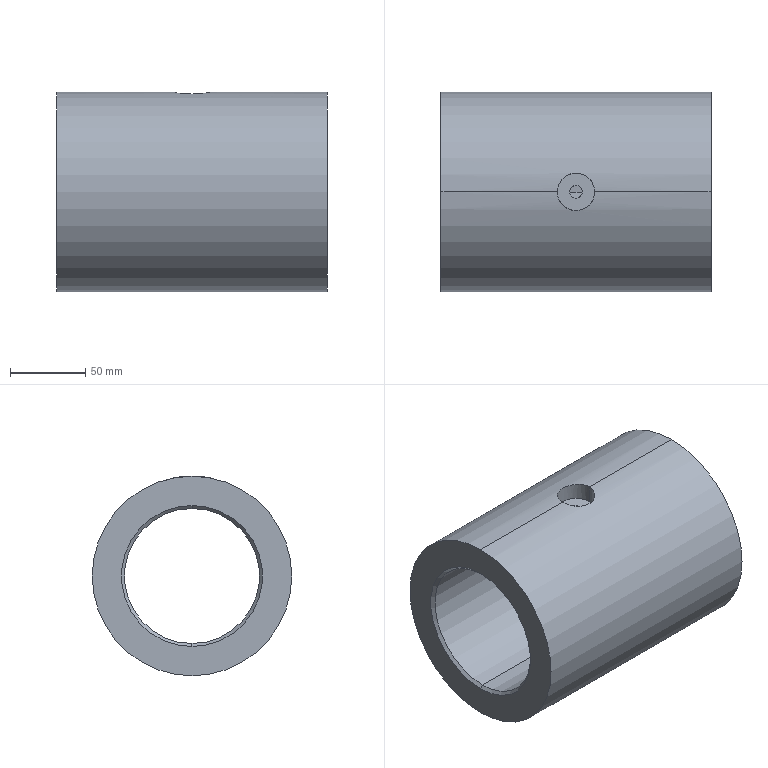Part | SolidWorks | features Chamfer 1, Extrusion 1, HoleWzd 1, ICE 1 | 1 solid | 15 faces | box 180 x 133 x 133 mm | volume 1348176 mm3 | cylinder 8 | cone 4 | plane 3 | commonest cylinder face diameters 8.5 x2 25 x2 90 x2 133 x2
STEP:
#1=CARTESIAN_POINT('',(88.,0.,45.));
#2=VERTEX_POINT('',#1);
#3=CARTESIAN_POINT('',(88.,0.,-45.));
#4=VERTEX_POINT('',#3);
#5=CARTESIAN_POINT('',(88.,0.,0.));
#6=DIRECTION('',(1.,0.,0.));
#7=DIRECTION('',(0.,0.,-1.));
#8=AXIS2_PLACEMENT_3D('',#5,#6,#7);
#9=CIRCLE('',#8,45.);
#10=EDGE_CURVE('',#2,#4,#9,.T.);
#11=ORIENTED_EDGE('',*,*,#10,.F.);
#12=CARTESIAN_POINT('',(90.,0.,47.));
#13=VERTEX_POINT('',#12);
#14=CARTESIAN_POINT('',(88.,0.,45.));
#15=DIRECTION('',(0.7071,0.,0.7071));
#16=VECTOR('',#15,1000.);
#17=LINE('',#14,#16);
#18=EDGE_CURVE('',#2,#13,#17,.T.);
#19=ORIENTED_EDGE('',*,*,#18,.T.);
#20=CARTESIAN_POINT('',(90.,0.,-47.));
#21=VERTEX_POINT('',#20);
#22=CARTESIAN_POINT('',(90.,0.,0.));
#23=DIRECTION('',(-1.,0.,0.));
#24=DIRECTION('',(0.,0.,-1.));
#25=AXIS2_PLACEMENT_3D('',#22,#23,#24);
#26=CIRCLE('',#25,47.);
#27=EDGE_CURVE('',#21,#13,#26,.T.);
#28=ORIENTED_EDGE('',*,*,#27,.F.);
#29=CARTESIAN_POINT('',(88.,0.,-45.));
#30=DIRECTION('',(0.7071,0.,-0.7071));
#31=VECTOR('',#30,1000.);
#32=LINE('',#29,#31);
#33=EDGE_CURVE('',#4,#21,#32,.T.);
#34=ORIENTED_EDGE('',*,*,#33,.F.);
#35=EDGE_LOOP('',(#11,#19,#28,#34));
#36=FACE_OUTER_BOUND('',#35,.T.);
#37=CARTESIAN_POINT('',(88.,0.,0.));
#38=DIRECTION('',(1.,0.,0.));
#39=DIRECTION('',(0.,0.,-1.));
#40=AXIS2_PLACEMENT_3D('',#37,#38,#39);
#41=CONICAL_SURFACE('',#40,45.,0.7854);
#42=ADVANCED_FACE('',(#36),#41,.F.);
#43=CARTESIAN_POINT('',(-88.,0.,-45.));
#44=VERTEX_POINT('',#43);
#45=CARTESIAN_POINT('',(-88.,0.,45.));
#46=VERTEX_POINT('',#45);
#47=CARTESIAN_POINT('',(-88.,0.,0.));
#48=DIRECTION('',(-1.,0.,0.));
#49=DIRECTION('',(0.,0.,-1.));
#50=AXIS2_PLACEMENT_3D('',#47,#48,#49);
#51=CIRCLE('',#50,45.);
#52=EDGE_CURVE('',#44,#46,#51,.T.);
#53=ORIENTED_EDGE('',*,*,#52,.F.);
#54=CARTESIAN_POINT('',(-90.,0.,-47.));
#55=VERTEX_POINT('',#54);
#56=CARTESIAN_POINT('',(-90.,0.,-47.));
#57=DIRECTION('',(-0.7071,0.,-0.7071));
#58=VECTOR('',#57,1000.);
#59=LINE('',#56,#58);
#60=EDGE_CURVE('',#44,#55,#59,.T.);
#61=ORIENTED_EDGE('',*,*,#60,.T.);
#62=CARTESIAN_POINT('',(-90.,0.,47.));
#63=VERTEX_POINT('',#62);
#64=CARTESIAN_POINT('',(-90.,0.,0.));
#65=DIRECTION('',(1.,0.,0.));
#66=DIRECTION('',(0.,0.,-1.));
#67=AXIS2_PLACEMENT_3D('',#64,#65,#66);
#68=CIRCLE('',#67,47.);
#69=EDGE_CURVE('',#63,#55,#68,.T.);
#70=ORIENTED_EDGE('',*,*,#69,.F.);
#71=CARTESIAN_POINT('',(-90.,0.,47.));
#72=DIRECTION('',(-0.7071,0.,0.7071));
#73=VECTOR('',#72,1000.);
#74=LINE('',#71,#73);
#75=EDGE_CURVE('',#46,#63,#74,.T.);
#76=ORIENTED_EDGE('',*,*,#75,.F.);
#77=EDGE_LOOP('',(#53,#61,#70,#76));
#78=FACE_OUTER_BOUND('',#77,.T.);
#79=CARTESIAN_POINT('',(-90.,0.,0.));
#80=DIRECTION('',(-1.,0.,0.));
#81=DIRECTION('',(0.,0.,1.));
#82=AXIS2_PLACEMENT_3D('',#79,#80,#81);
#83=CONICAL_SURFACE('',#82,47.,0.7854);
#84=ADVANCED_FACE('',(#78),#83,.F.);
#85=CARTESIAN_POINT('',(-12.5,0.,54.5));
#86=VERTEX_POINT('',#85);
#87=CARTESIAN_POINT('',(12.5,0.,54.5));
#88=VERTEX_POINT('',#87);
#89=CARTESIAN_POINT('',(0.,0.,54.5));
#90=DIRECTION('',(0.,0.,1.));
#91=DIRECTION('',(1.,0.,0.));
#92=AXIS2_PLACEMENT_3D('',#89,#90,#91);
#93=CIRCLE('',#92,12.5);
#94=EDGE_CURVE('',#86,#88,#93,.T.);
#95=ORIENTED_EDGE('',*,*,#94,.F.);
#96=CARTESIAN_POINT('',(-12.5,0.,66.5));
#97=VERTEX_POINT('',#96);
#98=CARTESIAN_POINT('',(-12.5,0.,54.5));
#99=DIRECTION('',(0.,0.,1.));
#100=VECTOR('',#99,1000.);
#101=LINE('',#98,#100);
#102=EDGE_CURVE('',#86,#97,#101,.T.);
#103=ORIENTED_EDGE('',*,*,#102,.T.);
#104=CARTESIAN_POINT('',(12.5,0.,66.5));
#105=VERTEX_POINT('',#104);
#106=CARTESIAN_POINT('',(12.5,0.,66.5));
#107=CARTESIAN_POINT('',(12.5,-0.8279,66.5));
#108=CARTESIAN_POINT('',(12.419,-1.642,66.485));
#109=CARTESIAN_POINT('',(12.18,-2.842,66.44));
#110=CARTESIAN_POINT('',(12.08,-3.238,66.422));
#111=CARTESIAN_POINT('',(11.841,-4.025,66.379));
#112=CARTESIAN_POINT('',(11.701,-4.415,66.354));
#113=CARTESIAN_POINT('',(11.23,-5.55,66.272));
#114=CARTESIAN_POINT('',(10.846,-6.267,66.208));
#115=CARTESIAN_POINT('',(10.166,-7.285,66.101));
#116=CARTESIAN_POINT('',(9.92,-7.616,66.063));
#117=CARTESIAN_POINT('',(9.399,-8.251,65.987));
#118=CARTESIAN_POINT('',(9.124,-8.553,65.948));
#119=CARTESIAN_POINT('',(8.261,-9.416,65.833));
#120=CARTESIAN_POINT('',(7.633,-9.933,65.756));
#121=CARTESIAN_POINT('',(6.609,-10.618,65.647));
#122=CARTESIAN_POINT('',(6.255,-10.83,65.612));
#123=CARTESIAN_POINT('',(5.535,-11.215,65.548));
#124=CARTESIAN_POINT('',(5.167,-11.39,65.518));
#125=CARTESIAN_POINT('',(4.415,-11.702,65.463));
#126=CARTESIAN_POINT('',(4.031,-11.839,65.438));
#127=CARTESIAN_POINT('',(3.248,-12.078,65.394));
#128=CARTESIAN_POINT('',(2.845,-12.179,65.375));
#129=CARTESIAN_POINT('',(1.635,-12.42,65.33));
#130=CARTESIAN_POINT('',(0.8222,-12.5,65.315));
#131=CARTESIAN_POINT('',(-0.4038,-12.5,65.315));
#132=CARTESIAN_POINT('',(-0.8137,-12.48,65.318));
#133=CARTESIAN_POINT('',(-1.636,-12.399,65.334));
#134=CARTESIAN_POINT('',(-2.044,-12.339,65.345));
#135=CARTESIAN_POINT('',(-3.248,-12.098,65.39));
#136=CARTESIAN_POINT('',(-4.028,-11.862,65.434));
#137=CARTESIAN_POINT('',(-5.164,-11.391,65.517));
#138=CARTESIAN_POINT('',(-5.539,-11.213,65.548));
#139=CARTESIAN_POINT('',(-6.261,-10.827,65.613));
#140=CARTESIAN_POINT('',(-6.61,-10.617,65.647));
#141=CARTESIAN_POINT('',(-7.287,-10.165,65.719));
#142=CARTESIAN_POINT('',(-7.613,-9.922,65.756));
#143=CARTESIAN_POINT('',(-8.244,-9.405,65.832));
#144=CARTESIAN_POINT('',(-8.549,-9.129,65.871));
#145=CARTESIAN_POINT('',(-9.421,-8.257,65.988));
#146=CARTESIAN_POINT('',(-9.936,-7.628,66.065));
#147=CARTESIAN_POINT('',(-10.615,-6.613,66.171));
#148=CARTESIAN_POINT('',(-10.825,-6.264,66.205));
#149=CARTESIAN_POINT('',(-11.213,-5.54,66.27));
#150=CARTESIAN_POINT('',(-11.39,-5.166,66.3));
#151=CARTESIAN_POINT('',(-11.86,-4.032,66.382));
#152=CARTESIAN_POINT('',(-12.097,-3.253,66.425));
#153=CARTESIAN_POINT('',(-12.338,-2.048,66.47));
#154=CARTESIAN_POINT('',(-12.399,-1.638,66.481));
#155=CARTESIAN_POINT('',(-12.48,-0.8177,66.496));
#156=CARTESIAN_POINT('',(-12.5,-0.4084,66.5));
#157=CARTESIAN_POINT('',(-12.5,0.,66.5));
#158=B_SPLINE_CURVE_WITH_KNOTS('',3,(#106,#107,#108,#109,#110,#111,#112,#113,#114,#115,#116,#117,#118,#119,#120,#121,#122,#123,#124,#125,#126,#127,#128,#129,#130,#131,#132,#133,#134,#135,#136,#137,#138,#139,#140,#141,#142,#143,#144,#145,#146,#147,#148,#149,#150,#151,#152,#153,#154,#155,#156,#157),.UNSPECIFIED.,.F.,.F.,(4,2,2,2,2,2,2,2,2,2,2,2,2,2,2,2,2,2,2,2,2,2,2,2,2,4),(0.,0.002448,0.003672,0.004896,0.007344,0.008568,0.009792,0.01224,0.01346,0.01469,0.01591,0.01714,0.01958,0.02081,0.02203,0.02448,0.0257,0.02693,0.02815,0.02938,0.03182,0.03305,0.03427,0.03672,0.03794,0.03917),.UNSPECIFIED.);
#159=EDGE_CURVE('',#105,#97,#158,.T.);
#160=ORIENTED_EDGE('',*,*,#159,.F.);
#161=CARTESIAN_POINT('',(12.5,0.,54.5));
#162=DIRECTION('',(0.,0.,1.));
#163=VECTOR('',#162,1000.);
#164=LINE('',#161,#163);
#165=EDGE_CURVE('',#88,#105,#164,.T.);
#166=ORIENTED_EDGE('',*,*,#165,.F.);
#167=EDGE_LOOP('',(#95,#103,#160,#166));
#168=FACE_OUTER_BOUND('',#167,.T.);
#169=CARTESIAN_POINT('',(0.,0.,54.5));
#170=DIRECTION('',(0.,0.,1.));
#171=DIRECTION('',(1.,0.,0.));
#172=AXIS2_PLACEMENT_3D('',#169,#170,#171);
#173=CYLINDRICAL_SURFACE('',#172,12.5);
#174=ADVANCED_FACE('',(#168),#173,.F.);
#175=ORIENTED_EDGE('',*,*,#10,.T.);
#176=CARTESIAN_POINT('',(90.,0.,-45.));
#177=DIRECTION('',(-1.,0.,0.));
#178=VECTOR('',#177,1000.);
#179=LINE('',#176,#178);
#180=EDGE_CURVE('',#4,#44,#179,.T.);
#181=ORIENTED_EDGE('',*,*,#180,.T.);
#182=ORIENTED_EDGE('',*,*,#52,.T.);
#183=CARTESIAN_POINT('',(-4.25,0.,45.));
#184=VERTEX_POINT('',#183);
#185=CARTESIAN_POINT('',(90.,0.,45.));
#186=DIRECTION('',(-1.,0.,0.));
#187=VECTOR('',#186,1000.);
#188=LINE('',#185,#187);
#189=EDGE_CURVE('',#184,#46,#188,.T.);
#190=ORIENTED_EDGE('',*,*,#189,.F.);
#191=CARTESIAN_POINT('',(4.25,0.,45.));
#192=VERTEX_POINT('',#191);
#193=CARTESIAN_POINT('',(4.25,0.,45.));
#194=CARTESIAN_POINT('',(4.25,-0.281,45.));
#195=CARTESIAN_POINT('',(4.222,-0.5572,44.997));
#196=CARTESIAN_POINT('',(4.114,-1.101,44.987));
#197=CARTESIAN_POINT('',(4.033,-1.371,44.98));
#198=CARTESIAN_POINT('',(3.819,-1.885,44.961));
#199=CARTESIAN_POINT('',(3.689,-2.129,44.95));
#200=CARTESIAN_POINT('',(3.38,-2.591,44.926));
#201=CARTESIAN_POINT('',(3.201,-2.81,44.913));
#202=CARTESIAN_POINT('',(2.809,-3.202,44.886));
#203=CARTESIAN_POINT('',(2.595,-3.378,44.873));
#204=CARTESIAN_POINT('',(2.13,-3.688,44.849));
#205=CARTESIAN_POINT('',(1.883,-3.82,44.838));
#206=CARTESIAN_POINT('',(1.372,-4.032,44.819));
#207=CARTESIAN_POINT('',(1.104,-4.114,44.812));
#208=CARTESIAN_POINT('',(0.5548,-4.223,44.801));
#209=CARTESIAN_POINT('',(0.2789,-4.25,44.799));
#210=CARTESIAN_POINT('',(-0.2758,-4.25,44.799));
#211=CARTESIAN_POINT('',(-0.5576,-4.222,44.801));
#212=CARTESIAN_POINT('',(-1.103,-4.114,44.812));
#213=CARTESIAN_POINT('',(-1.368,-4.034,44.819));
#214=CARTESIAN_POINT('',(-1.883,-3.82,44.838));
#215=CARTESIAN_POINT('',(-2.131,-3.687,44.849));
#216=CARTESIAN_POINT('',(-2.592,-3.38,44.873));
#217=CARTESIAN_POINT('',(-2.806,-3.204,44.886));
#218=CARTESIAN_POINT('',(-3.203,-2.807,44.913));
#219=CARTESIAN_POINT('',(-3.379,-2.593,44.926));
#220=CARTESIAN_POINT('',(-3.687,-2.132,44.95));
#221=CARTESIAN_POINT('',(-3.82,-1.884,44.961));
#222=CARTESIAN_POINT('',(-4.033,-1.369,44.98));
#223=CARTESIAN_POINT('',(-4.113,-1.104,44.987));
#224=CARTESIAN_POINT('',(-4.222,-0.5593,44.997));
#225=CARTESIAN_POINT('',(-4.25,-0.2775,45.));
#226=CARTESIAN_POINT('',(-4.25,0.,45.));
#227=B_SPLINE_CURVE_WITH_KNOTS('',3,(#193,#194,#195,#196,#197,#198,#199,#200,#201,#202,#203,#204,#205,#206,#207,#208,#209,#210,#211,#212,#213,#214,#215,#216,#217,#218,#219,#220,#221,#222,#223,#224,#225,#226),.UNSPECIFIED.,.F.,.F.,(4,2,2,2,2,2,2,2,2,2,2,2,2,2,2,2,4),(0.,0.0008309,0.001662,0.002493,0.003324,0.004155,0.004986,0.005816,0.006647,0.007478,0.008309,0.00914,0.009971,0.0108,0.01163,0.01246,0.01329),.UNSPECIFIED.);
#228=EDGE_CURVE('',#192,#184,#227,.T.);
#229=ORIENTED_EDGE('',*,*,#228,.F.);
#230=CARTESIAN_POINT('',(90.,0.,45.));
#231=DIRECTION('',(-1.,0.,0.));
#232=VECTOR('',#231,1000.);
#233=LINE('',#230,#232);
#234=EDGE_CURVE('',#2,#192,#233,.T.);
#235=ORIENTED_EDGE('',*,*,#234,.F.);
#236=EDGE_LOOP('',(#175,#181,#182,#190,#229,#235));
#237=FACE_OUTER_BOUND('',#236,.T.);
#238=CARTESIAN_POINT('',(90.,0.,0.));
#239=DIRECTION('',(-1.,0.,0.));
#240=DIRECTION('',(0.,0.,1.));
#241=AXIS2_PLACEMENT_3D('',#238,#239,#240);
#242=CYLINDRICAL_SURFACE('',#241,45.);
#243=ADVANCED_FACE('',(#237),#242,.F.);
#244=CARTESIAN_POINT('',(90.,0.,-66.5));
#245=VERTEX_POINT('',#244);
#246=CARTESIAN_POINT('',(90.,0.,66.5));
#247=VERTEX_POINT('',#246);
#248=CARTESIAN_POINT('',(90.,0.,0.));
#249=DIRECTION('',(1.,0.,0.));
#250=DIRECTION('',(0.,0.,-1.));
#251=AXIS2_PLACEMENT_3D('',#248,#249,#250);
#252=CIRCLE('',#251,66.5);
#253=EDGE_CURVE('',#245,#247,#252,.T.);
#254=ORIENTED_EDGE('',*,*,#253,.F.);
#255=CARTESIAN_POINT('',(-90.,0.,-66.5));
#256=VERTEX_POINT('',#255);
#257=CARTESIAN_POINT('',(90.,0.,-66.5));
#258=DIRECTION('',(-1.,0.,0.));
#259=VECTOR('',#258,1000.);
#260=LINE('',#257,#259);
#261=EDGE_CURVE('',#245,#256,#260,.T.);
#262=ORIENTED_EDGE('',*,*,#261,.T.);
#263=CARTESIAN_POINT('',(-90.,0.,66.5));
#264=VERTEX_POINT('',#263);
#265=CARTESIAN_POINT('',(-90.,0.,0.));
#266=DIRECTION('',(1.,0.,0.));
#267=DIRECTION('',(0.,0.,-1.));
#268=AXIS2_PLACEMENT_3D('',#265,#266,#267);
#269=CIRCLE('',#268,66.5);
#270=EDGE_CURVE('',#256,#264,#269,.T.);
#271=ORIENTED_EDGE('',*,*,#270,.T.);
#272=CARTESIAN_POINT('',(90.,0.,66.5));
#273=DIRECTION('',(-1.,0.,0.));
#274=VECTOR('',#273,1000.);
#275=LINE('',#272,#274);
#276=EDGE_CURVE('',#97,#264,#275,.T.);
#277=ORIENTED_EDGE('',*,*,#276,.F.);
#278=CARTESIAN_POINT('',(-12.5,0.,66.5));
#279=CARTESIAN_POINT('',(-12.5,0.8166,66.5));
#280=CARTESIAN_POINT('',(-12.421,1.629,66.485));
#281=CARTESIAN_POINT('',(-12.179,2.843,66.44));
#282=CARTESIAN_POINT('',(-12.079,3.244,66.422));
#283=CARTESIAN_POINT('',(-11.841,4.026,66.379));
#284=CARTESIAN_POINT('',(-11.703,4.41,66.355));
#285=CARTESIAN_POINT('',(-11.392,5.162,66.3));
#286=CARTESIAN_POINT('',(-11.217,5.531,66.271));
#287=CARTESIAN_POINT('',(-10.831,6.253,66.206));
#288=CARTESIAN_POINT('',(-10.618,6.608,66.172));
#289=CARTESIAN_POINT('',(-9.936,7.629,66.064));
#290=CARTESIAN_POINT('',(-9.42,8.257,65.988));
#291=CARTESIAN_POINT('',(-8.556,9.122,65.872));
#292=CARTESIAN_POINT('',(-8.253,9.398,65.833));
#293=CARTESIAN_POINT('',(-7.617,9.92,65.756));
#294=CARTESIAN_POINT('',(-7.288,10.163,65.719));
#295=CARTESIAN_POINT('',(-6.273,10.843,65.612));
#296=CARTESIAN_POINT('',(-5.556,11.227,65.546));
#297=CARTESIAN_POINT('',(-4.419,11.7,65.463));
#298=CARTESIAN_POINT('',(-4.029,11.84,65.438));
#299=CARTESIAN_POINT('',(-3.245,12.078,65.394));
#300=CARTESIAN_POINT('',(-2.454,12.277,65.357));
#301=CARTESIAN_POINT('',(-1.647,12.398,65.334));
#302=CARTESIAN_POINT('',(-0.8324,12.479,65.319));
#303=CARTESIAN_POINT('',(-0.4195,12.5,65.315));
#304=CARTESIAN_POINT('',(0.8187,12.5,65.315));
#305=CARTESIAN_POINT('',(1.632,12.42,65.33));
#306=CARTESIAN_POINT('',(2.833,12.182,65.375));
#307=CARTESIAN_POINT('',(3.23,12.083,65.393));
#308=CARTESIAN_POINT('',(4.018,11.844,65.437));
#309=CARTESIAN_POINT('',(4.407,11.704,65.462));
#310=CARTESIAN_POINT('',(5.54,11.235,65.545));
#311=CARTESIAN_POINT('',(6.258,10.852,65.61));
#312=CARTESIAN_POINT('',(7.278,10.171,65.718));
#313=CARTESIAN_POINT('',(7.61,9.925,65.756));
#314=CARTESIAN_POINT('',(8.244,9.405,65.832));
#315=CARTESIAN_POINT('',(8.546,9.132,65.871));
#316=CARTESIAN_POINT('',(9.408,8.27,65.986));
#317=CARTESIAN_POINT('',(9.926,7.642,66.063));
#318=CARTESIAN_POINT('',(10.843,6.273,66.207));
#319=CARTESIAN_POINT('',(11.228,5.554,66.272));
#320=CARTESIAN_POINT('',(11.697,4.426,66.354));
#321=CARTESIAN_POINT('',(11.835,4.042,66.378));
#322=CARTESIAN_POINT('',(12.075,3.257,66.421));
#323=CARTESIAN_POINT('',(12.177,2.855,66.44));
#324=CARTESIAN_POINT('',(12.419,1.645,66.485));
#325=CARTESIAN_POINT('',(12.5,0.8277,66.5));
#326=CARTESIAN_POINT('',(12.5,0.,66.5));
#327=B_SPLINE_CURVE_WITH_KNOTS('',3,(#278,#279,#280,#281,#282,#283,#284,#285,#286,#287,#288,#289,#290,#291,#292,#293,#294,#295,#296,#297,#298,#299,#300,#301,#302,#303,#304,#305,#306,#307,#308,#309,#310,#311,#312,#313,#314,#315,#316,#317,#318,#319,#320,#321,#322,#323,#324,#325,#326),.UNSPECIFIED.,.F.,.F.,(4,2,2,2,2,2,2,2,2,2,2,1,2,2,2,2,2,2,2,2,2,2,2,2,4),(0.03917,0.04162,0.04284,0.04406,0.04529,0.04651,0.04896,0.05018,0.0514,0.05385,0.05508,0.0563,0.05752,0.05875,0.06119,0.06242,0.06364,0.06609,0.06731,0.06854,0.07098,0.07343,0.07465,0.07588,0.07833),.UNSPECIFIED.);
#328=EDGE_CURVE('',#97,#105,#327,.T.);
#329=ORIENTED_EDGE('',*,*,#328,.T.);
#330=CARTESIAN_POINT('',(90.,0.,66.5));
#331=DIRECTION('',(-1.,0.,0.));
#332=VECTOR('',#331,1000.);
#333=LINE('',#330,#332);
#334=EDGE_CURVE('',#247,#105,#333,.T.);
#335=ORIENTED_EDGE('',*,*,#334,.F.);
#336=EDGE_LOOP('',(#254,#262,#271,#277,#329,#335));
#337=FACE_OUTER_BOUND('',#336,.T.);
#338=CARTESIAN_POINT('',(90.,0.,0.));
#339=DIRECTION('',(-1.,0.,0.));
#340=DIRECTION('',(0.,0.,1.));
#341=AXIS2_PLACEMENT_3D('',#338,#339,#340);
#342=CYLINDRICAL_SURFACE('',#341,66.5);
#343=ADVANCED_FACE('',(#337),#342,.T.);
#344=ORIENTED_EDGE('',*,*,#228,.T.);
#345=CARTESIAN_POINT('',(-4.25,0.,54.5));
#346=VERTEX_POINT('',#345);
#347=CARTESIAN_POINT('',(-4.25,0.,66.5));
#348=DIRECTION('',(0.,0.,1.));
#349=VECTOR('',#348,1000.);
#350=LINE('',#347,#349);
#351=EDGE_CURVE('',#184,#346,#350,.T.);
#352=ORIENTED_EDGE('',*,*,#351,.T.);
#353=CARTESIAN_POINT('',(4.25,0.,54.5));
#354=VERTEX_POINT('',#353);
#355=CARTESIAN_POINT('',(0.,0.,54.5));
#356=DIRECTION('',(0.,0.,-1.));
#357=DIRECTION('',(1.,0.,0.));
#358=AXIS2_PLACEMENT_3D('',#355,#356,#357);
#359=CIRCLE('',#358,4.25);
#360=EDGE_CURVE('',#354,#346,#359,.T.);
#361=ORIENTED_EDGE('',*,*,#360,.F.);
#362=CARTESIAN_POINT('',(4.25,0.,66.5));
#363=DIRECTION('',(0.,0.,1.));
#364=VECTOR('',#363,1000.);
#365=LINE('',#362,#364);
#366=EDGE_CURVE('',#192,#354,#365,.T.);
#367=ORIENTED_EDGE('',*,*,#366,.F.);
#368=EDGE_LOOP('',(#344,#352,#361,#367));
#369=FACE_OUTER_BOUND('',#368,.T.);
#370=CARTESIAN_POINT('',(0.,0.,66.5));
#371=DIRECTION('',(0.,0.,1.));
#372=DIRECTION('',(1.,0.,0.));
#373=AXIS2_PLACEMENT_3D('',#370,#371,#372);
#374=CYLINDRICAL_SURFACE('',#373,4.25);
#375=ADVANCED_FACE('',(#369),#374,.F.);
#376=ORIENTED_EDGE('',*,*,#351,.F.);
#377=CARTESIAN_POINT('',(-4.25,0.,45.));
#378=CARTESIAN_POINT('',(-4.25,0.2774,45.));
#379=CARTESIAN_POINT('',(-4.223,0.5532,44.997));
#380=CARTESIAN_POINT('',(-4.114,1.102,44.987));
#381=CARTESIAN_POINT('',(-4.033,1.37,44.98));
#382=CARTESIAN_POINT('',(-3.821,1.881,44.961));
#383=CARTESIAN_POINT('',(-3.689,2.128,44.95));
#384=CARTESIAN_POINT('',(-3.379,2.593,44.926));
#385=CARTESIAN_POINT('',(-3.203,2.807,44.913));
#386=CARTESIAN_POINT('',(-2.812,3.199,44.887));
#387=CARTESIAN_POINT('',(-2.593,3.379,44.873));
#388=CARTESIAN_POINT('',(-2.131,3.687,44.849));
#389=CARTESIAN_POINT('',(-1.888,3.818,44.838));
#390=CARTESIAN_POINT('',(-1.373,4.032,44.819));
#391=CARTESIAN_POINT('',(-1.103,4.114,44.812));
#392=CARTESIAN_POINT('',(-0.5601,4.222,44.802));
#393=CARTESIAN_POINT('',(-0.284,4.25,44.799));
#394=CARTESIAN_POINT('',(0.2774,4.25,44.799));
#395=CARTESIAN_POINT('',(0.5541,4.223,44.801));
#396=CARTESIAN_POINT('',(1.097,4.115,44.811));
#397=CARTESIAN_POINT('',(1.367,4.034,44.819));
#398=CARTESIAN_POINT('',(1.882,3.821,44.838));
#399=CARTESIAN_POINT('',(2.126,3.69,44.849));
#400=CARTESIAN_POINT('',(2.588,3.382,44.873));
#401=CARTESIAN_POINT('',(2.807,3.203,44.886));
#402=CARTESIAN_POINT('',(3.199,2.811,44.913));
#403=CARTESIAN_POINT('',(3.375,2.598,44.926));
#404=CARTESIAN_POINT('',(3.686,2.134,44.95));
#405=CARTESIAN_POINT('',(3.818,1.887,44.961));
#406=CARTESIAN_POINT('',(4.031,1.376,44.98));
#407=CARTESIAN_POINT('',(4.113,1.108,44.987));
#408=CARTESIAN_POINT('',(4.222,0.5587,44.997));
#409=CARTESIAN_POINT('',(4.25,0.2809,45.));
#410=CARTESIAN_POINT('',(4.25,0.,45.));
#411=B_SPLINE_CURVE_WITH_KNOTS('',3,(#377,#378,#379,#380,#381,#382,#383,#384,#385,#386,#387,#388,#389,#390,#391,#392,#393,#394,#395,#396,#397,#398,#399,#400,#401,#402,#403,#404,#405,#406,#407,#408,#409,#410),.UNSPECIFIED.,.F.,.F.,(4,2,2,2,2,2,2,2,2,2,2,2,2,2,2,2,4),(0.01329,0.01413,0.01496,0.01579,0.01662,0.01745,0.01828,0.01911,0.01994,0.02077,0.0216,0.02243,0.02326,0.02409,0.02493,0.02576,0.02659),.UNSPECIFIED.);
#412=EDGE_CURVE('',#184,#192,#411,.T.);
#413=ORIENTED_EDGE('',*,*,#412,.T.);
#414=ORIENTED_EDGE('',*,*,#366,.T.);
#415=CARTESIAN_POINT('',(0.,0.,54.5));
#416=DIRECTION('',(0.,0.,-1.));
#417=DIRECTION('',(1.,0.,0.));
#418=AXIS2_PLACEMENT_3D('',#415,#416,#417);
#419=CIRCLE('',#418,4.25);
#420=EDGE_CURVE('',#346,#354,#419,.T.);
#421=ORIENTED_EDGE('',*,*,#420,.F.);
#422=EDGE_LOOP('',(#376,#413,#414,#421));
#423=FACE_OUTER_BOUND('',#422,.T.);
#424=CARTESIAN_POINT('',(0.,0.,66.5));
#425=DIRECTION('',(0.,0.,1.));
#426=DIRECTION('',(1.,0.,0.));
#427=AXIS2_PLACEMENT_3D('',#424,#425,#426);
#428=CYLINDRICAL_SURFACE('',#427,4.25);
#429=ADVANCED_FACE('',(#423),#428,.F.);
#430=ORIENTED_EDGE('',*,*,#27,.T.);
#431=CARTESIAN_POINT('',(90.,0.,0.));
#432=DIRECTION('',(-1.,0.,0.));
#433=DIRECTION('',(0.,0.,-1.));
#434=AXIS2_PLACEMENT_3D('',#431,#432,#433);
#435=CIRCLE('',#434,47.);
#436=EDGE_CURVE('',#13,#21,#435,.T.);
#437=ORIENTED_EDGE('',*,*,#436,.T.);
#438=EDGE_LOOP('',(#430,#437));
#439=FACE_BOUND('',#438,.T.);
#440=CARTESIAN_POINT('',(90.,0.,0.));
#441=DIRECTION('',(1.,0.,0.));
#442=DIRECTION('',(0.,0.,-1.));
#443=AXIS2_PLACEMENT_3D('',#440,#441,#442);
#444=CIRCLE('',#443,66.5);
#445=EDGE_CURVE('',#247,#245,#444,.T.);
#446=ORIENTED_EDGE('',*,*,#445,.T.);
#447=ORIENTED_EDGE('',*,*,#253,.T.);
#448=EDGE_LOOP('',(#446,#447));
#449=FACE_OUTER_BOUND('',#448,.T.);
#450=CARTESIAN_POINT('',(90.,0.,0.));
#451=DIRECTION('',(1.,0.,0.));
#452=DIRECTION('',(0.,0.,-1.));
#453=AXIS2_PLACEMENT_3D('',#450,#451,#452);
#454=PLANE('',#453);
#455=ADVANCED_FACE('',(#439,#449),#454,.T.);
#456=ORIENTED_EDGE('',*,*,#69,.T.);
#457=CARTESIAN_POINT('',(-90.,0.,0.));
#458=DIRECTION('',(1.,0.,0.));
#459=DIRECTION('',(0.,0.,-1.));
#460=AXIS2_PLACEMENT_3D('',#457,#458,#459);
#461=CIRCLE('',#460,47.);
#462=EDGE_CURVE('',#55,#63,#461,.T.);
#463=ORIENTED_EDGE('',*,*,#462,.T.);
#464=EDGE_LOOP('',(#456,#463));
#465=FACE_BOUND('',#464,.T.);
#466=CARTESIAN_POINT('',(-90.,0.,0.));
#467=DIRECTION('',(1.,0.,0.));
#468=DIRECTION('',(0.,0.,-1.));
#469=AXIS2_PLACEMENT_3D('',#466,#467,#468);
#470=CIRCLE('',#469,66.5);
#471=EDGE_CURVE('',#264,#256,#470,.T.);
#472=ORIENTED_EDGE('',*,*,#471,.F.);
#473=ORIENTED_EDGE('',*,*,#270,.F.);
#474=EDGE_LOOP('',(#472,#473));
#475=FACE_OUTER_BOUND('',#474,.T.);
#476=CARTESIAN_POINT('',(-90.,0.,0.));
#477=DIRECTION('',(1.,0.,0.));
#478=DIRECTION('',(0.,0.,-1.));
#479=AXIS2_PLACEMENT_3D('',#476,#477,#478);
#480=PLANE('',#479);
#481=ADVANCED_FACE('',(#465,#475),#480,.F.);
#482=ORIENTED_EDGE('',*,*,#261,.F.);
#483=ORIENTED_EDGE('',*,*,#445,.F.);
#484=ORIENTED_EDGE('',*,*,#334,.T.);
#485=ORIENTED_EDGE('',*,*,#159,.T.);
#486=ORIENTED_EDGE('',*,*,#276,.T.);
#487=ORIENTED_EDGE('',*,*,#471,.T.);
#488=EDGE_LOOP('',(#482,#483,#484,#485,#486,#487));
#489=FACE_OUTER_BOUND('',#488,.T.);
#490=CARTESIAN_POINT('',(90.,0.,0.));
#491=DIRECTION('',(-1.,0.,0.));
#492=DIRECTION('',(0.,0.,1.));
#493=AXIS2_PLACEMENT_3D('',#490,#491,#492);
#494=CYLINDRICAL_SURFACE('',#493,66.5);
#495=ADVANCED_FACE('',(#489),#494,.T.);
#496=ORIENTED_EDGE('',*,*,#180,.F.);
#497=CARTESIAN_POINT('',(88.,0.,0.));
#498=DIRECTION('',(1.,0.,0.));
#499=DIRECTION('',(0.,0.,-1.));
#500=AXIS2_PLACEMENT_3D('',#497,#498,#499);
#501=CIRCLE('',#500,45.);
#502=EDGE_CURVE('',#4,#2,#501,.T.);
#503=ORIENTED_EDGE('',*,*,#502,.T.);
#504=ORIENTED_EDGE('',*,*,#234,.T.);
#505=ORIENTED_EDGE('',*,*,#412,.F.);
#506=ORIENTED_EDGE('',*,*,#189,.T.);
#507=CARTESIAN_POINT('',(-88.,0.,0.));
#508=DIRECTION('',(-1.,0.,0.));
#509=DIRECTION('',(0.,0.,-1.));
#510=AXIS2_PLACEMENT_3D('',#507,#508,#509);
#511=CIRCLE('',#510,45.);
#512=EDGE_CURVE('',#46,#44,#511,.T.);
#513=ORIENTED_EDGE('',*,*,#512,.T.);
#514=EDGE_LOOP('',(#496,#503,#504,#505,#506,#513));
#515=FACE_OUTER_BOUND('',#514,.T.);
#516=CARTESIAN_POINT('',(90.,0.,0.));
#517=DIRECTION('',(-1.,0.,0.));
#518=DIRECTION('',(0.,0.,1.));
#519=AXIS2_PLACEMENT_3D('',#516,#517,#518);
#520=CYLINDRICAL_SURFACE('',#519,45.);
#521=ADVANCED_FACE('',(#515),#520,.F.);
#522=ORIENTED_EDGE('',*,*,#102,.F.);
#523=CARTESIAN_POINT('',(0.,0.,54.5));
#524=DIRECTION('',(0.,0.,1.));
#525=DIRECTION('',(1.,0.,0.));
#526=AXIS2_PLACEMENT_3D('',#523,#524,#525);
#527=CIRCLE('',#526,12.5);
#528=EDGE_CURVE('',#88,#86,#527,.T.);
#529=ORIENTED_EDGE('',*,*,#528,.F.);
#530=ORIENTED_EDGE('',*,*,#165,.T.);
#531=ORIENTED_EDGE('',*,*,#328,.F.);
#532=EDGE_LOOP('',(#522,#529,#530,#531));
#533=FACE_OUTER_BOUND('',#532,.T.);
#534=CARTESIAN_POINT('',(0.,0.,54.5));
#535=DIRECTION('',(0.,0.,1.));
#536=DIRECTION('',(1.,0.,0.));
#537=AXIS2_PLACEMENT_3D('',#534,#535,#536);
#538=CYLINDRICAL_SURFACE('',#537,12.5);
#539=ADVANCED_FACE('',(#533),#538,.F.);
#540=ORIENTED_EDGE('',*,*,#528,.T.);
#541=ORIENTED_EDGE('',*,*,#94,.T.);
#542=EDGE_LOOP('',(#540,#541));
#543=FACE_OUTER_BOUND('',#542,.T.);
#544=ORIENTED_EDGE('',*,*,#360,.T.);
#545=ORIENTED_EDGE('',*,*,#420,.T.);
#546=EDGE_LOOP('',(#544,#545));
#547=FACE_BOUND('',#546,.T.);
#548=CARTESIAN_POINT('',(0.,0.,54.5));
#549=DIRECTION('',(0.,0.,1.));
#550=DIRECTION('',(1.,0.,0.));
#551=AXIS2_PLACEMENT_3D('',#548,#549,#550);
#552=PLANE('',#551);
#553=ADVANCED_FACE('',(#543,#547),#552,.T.);
#554=ORIENTED_EDGE('',*,*,#60,.F.);
#555=ORIENTED_EDGE('',*,*,#512,.F.);
#556=ORIENTED_EDGE('',*,*,#75,.T.);
#557=ORIENTED_EDGE('',*,*,#462,.F.);
#558=EDGE_LOOP('',(#554,#555,#556,#557));
#559=FACE_OUTER_BOUND('',#558,.T.);
#560=CARTESIAN_POINT('',(-90.,0.,0.));
#561=DIRECTION('',(-1.,0.,0.));
#562=DIRECTION('',(0.,0.,1.));
#563=AXIS2_PLACEMENT_3D('',#560,#561,#562);
#564=CONICAL_SURFACE('',#563,47.,0.7854);
#565=ADVANCED_FACE('',(#559),#564,.F.);
#566=ORIENTED_EDGE('',*,*,#18,.F.);
#567=ORIENTED_EDGE('',*,*,#502,.F.);
#568=ORIENTED_EDGE('',*,*,#33,.T.);
#569=ORIENTED_EDGE('',*,*,#436,.F.);
#570=EDGE_LOOP('',(#566,#567,#568,#569));
#571=FACE_OUTER_BOUND('',#570,.T.);
#572=CARTESIAN_POINT('',(88.,0.,0.));
#573=DIRECTION('',(1.,0.,0.));
#574=DIRECTION('',(0.,0.,-1.));
#575=AXIS2_PLACEMENT_3D('',#572,#573,#574);
#576=CONICAL_SURFACE('',#575,45.,0.7854);
#577=ADVANCED_FACE('',(#571),#576,.F.);
#578=CLOSED_SHELL('',(#42,#84,#174,#243,#343,#375,#429,#455,#481,#495,#521,#539,#553,#565,#577));
#579=MANIFOLD_SOLID_BREP('',#578);
#580=CARTESIAN_POINT('',(0.,0.,0.));
#581=DIRECTION('',(0.,0.,1.));
#582=DIRECTION('',(1.,0.,0.));
#583=AXIS2_PLACEMENT_3D('',#580,#581,#582);
#584=(LENGTH_UNIT()NAMED_UNIT(*)SI_UNIT(.MILLI.,.METRE.));
#585=UNCERTAINTY_MEASURE_WITH_UNIT(LENGTH_MEASURE(0.00001),#584,'','');
#586=(NAMED_UNIT(*)PLANE_ANGLE_UNIT()SI_UNIT($,.RADIAN.));
#587=(NAMED_UNIT(*)SI_UNIT($,.STERADIAN.)SOLID_ANGLE_UNIT());
#588=(GEOMETRIC_REPRESENTATION_CONTEXT(3)GLOBAL_UNCERTAINTY_ASSIGNED_CONTEXT((#585))GLOBAL_UNIT_ASSIGNED_CONTEXT((#584,#586,#587))REPRESENTATION_CONTEXT('',''));
#589=ADVANCED_BREP_SHAPE_REPRESENTATION('',(#579,#583),#588);